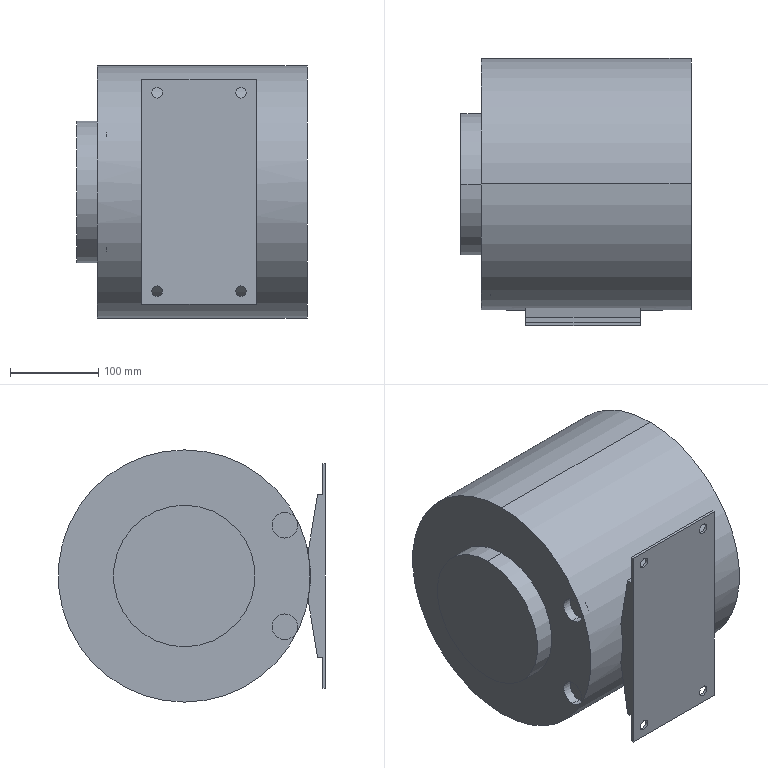Part | SolidWorks | features BaseBody 1 | 1 solid | 32 faces | box 261 x 303 x 286 mm | volume 16134970 mm3 | cylinder 16 | plane 16 | commonest cylinder face diameters 12 x8 28.835 x4 160.568 x2 286 x2
STEP:
#1=CARTESIAN_POINT('',(10.,-114.,-71.917));
#2=VERTEX_POINT('',#1);
#3=CARTESIAN_POINT('',(10.,-114.,-43.083));
#4=VERTEX_POINT('',#3);
#5=CARTESIAN_POINT('',(10.,-114.,-57.5));
#6=DIRECTION('',(-1.,0.,0.));
#7=DIRECTION('',(0.,0.,-1.));
#8=AXIS2_PLACEMENT_3D('',#5,#6,#7);
#9=CIRCLE('',#8,14.417);
#10=EDGE_CURVE('',#2,#4,#9,.T.);
#11=ORIENTED_EDGE('',*,*,#10,.F.);
#12=CARTESIAN_POINT('',(0.,-114.,-71.917));
#13=VERTEX_POINT('',#12);
#14=CARTESIAN_POINT('',(10.,-114.,-71.917));
#15=DIRECTION('',(-1.,0.,0.));
#16=VECTOR('',#15,1000.);
#17=LINE('',#14,#16);
#18=EDGE_CURVE('',#2,#13,#17,.T.);
#19=ORIENTED_EDGE('',*,*,#18,.T.);
#20=CARTESIAN_POINT('',(0.,-114.,-43.083));
#21=VERTEX_POINT('',#20);
#22=CARTESIAN_POINT('',(0.,-114.,-57.5));
#23=DIRECTION('',(-1.,0.,0.));
#24=DIRECTION('',(0.,0.,-1.));
#25=AXIS2_PLACEMENT_3D('',#22,#23,#24);
#26=CIRCLE('',#25,14.417);
#27=EDGE_CURVE('',#13,#21,#26,.T.);
#28=ORIENTED_EDGE('',*,*,#27,.T.);
#29=CARTESIAN_POINT('',(10.,-114.,-43.083));
#30=DIRECTION('',(-1.,0.,0.));
#31=VECTOR('',#30,1000.);
#32=LINE('',#29,#31);
#33=EDGE_CURVE('',#4,#21,#32,.T.);
#34=ORIENTED_EDGE('',*,*,#33,.F.);
#35=EDGE_LOOP('',(#11,#19,#28,#34));
#36=FACE_OUTER_BOUND('',#35,.T.);
#37=CARTESIAN_POINT('',(10.,-114.,-57.5));
#38=DIRECTION('',(-1.,0.,0.));
#39=DIRECTION('',(0.,0.,1.));
#40=AXIS2_PLACEMENT_3D('',#37,#38,#39);
#41=CYLINDRICAL_SURFACE('',#40,14.417);
#42=ADVANCED_FACE('',(#36),#41,.F.);
#43=CARTESIAN_POINT('',(10.,-114.,43.083));
#44=VERTEX_POINT('',#43);
#45=CARTESIAN_POINT('',(10.,-114.,71.917));
#46=VERTEX_POINT('',#45);
#47=CARTESIAN_POINT('',(10.,-114.,57.5));
#48=DIRECTION('',(-1.,0.,0.));
#49=DIRECTION('',(0.,0.,1.));
#50=AXIS2_PLACEMENT_3D('',#47,#48,#49);
#51=CIRCLE('',#50,14.417);
#52=EDGE_CURVE('',#44,#46,#51,.T.);
#53=ORIENTED_EDGE('',*,*,#52,.F.);
#54=CARTESIAN_POINT('',(0.,-114.,43.083));
#55=VERTEX_POINT('',#54);
#56=CARTESIAN_POINT('',(10.,-114.,43.083));
#57=DIRECTION('',(-1.,0.,0.));
#58=VECTOR('',#57,1000.);
#59=LINE('',#56,#58);
#60=EDGE_CURVE('',#44,#55,#59,.T.);
#61=ORIENTED_EDGE('',*,*,#60,.T.);
#62=CARTESIAN_POINT('',(0.,-114.,71.917));
#63=VERTEX_POINT('',#62);
#64=CARTESIAN_POINT('',(0.,-114.,57.5));
#65=DIRECTION('',(-1.,0.,0.));
#66=DIRECTION('',(0.,0.,1.));
#67=AXIS2_PLACEMENT_3D('',#64,#65,#66);
#68=CIRCLE('',#67,14.417);
#69=EDGE_CURVE('',#55,#63,#68,.T.);
#70=ORIENTED_EDGE('',*,*,#69,.T.);
#71=CARTESIAN_POINT('',(10.,-114.,71.917));
#72=DIRECTION('',(-1.,0.,0.));
#73=VECTOR('',#72,1000.);
#74=LINE('',#71,#73);
#75=EDGE_CURVE('',#46,#63,#74,.T.);
#76=ORIENTED_EDGE('',*,*,#75,.F.);
#77=EDGE_LOOP('',(#53,#61,#70,#76));
#78=FACE_OUTER_BOUND('',#77,.T.);
#79=CARTESIAN_POINT('',(10.,-114.,57.5));
#80=DIRECTION('',(-1.,0.,0.));
#81=DIRECTION('',(0.,0.,1.));
#82=AXIS2_PLACEMENT_3D('',#79,#80,#81);
#83=CYLINDRICAL_SURFACE('',#82,14.417);
#84=ADVANCED_FACE('',(#78),#83,.F.);
#85=CARTESIAN_POINT('',(-23.,0.,80.284));
#86=VERTEX_POINT('',#85);
#87=CARTESIAN_POINT('',(-23.,0.,-80.284));
#88=VERTEX_POINT('',#87);
#89=CARTESIAN_POINT('',(-23.,0.,0.));
#90=DIRECTION('',(-1.,0.,0.));
#91=DIRECTION('',(0.,0.,1.));
#92=AXIS2_PLACEMENT_3D('',#89,#90,#91);
#93=CIRCLE('',#92,80.284);
#94=EDGE_CURVE('',#86,#88,#93,.T.);
#95=ORIENTED_EDGE('',*,*,#94,.F.);
#96=CARTESIAN_POINT('',(0.,0.,80.284));
#97=VERTEX_POINT('',#96);
#98=CARTESIAN_POINT('',(-23.,0.,80.284));
#99=DIRECTION('',(1.,0.,0.));
#100=VECTOR('',#99,1000.);
#101=LINE('',#98,#100);
#102=EDGE_CURVE('',#86,#97,#101,.T.);
#103=ORIENTED_EDGE('',*,*,#102,.T.);
#104=CARTESIAN_POINT('',(0.,0.,-80.284));
#105=VERTEX_POINT('',#104);
#106=CARTESIAN_POINT('',(0.,0.,0.));
#107=DIRECTION('',(-1.,0.,0.));
#108=DIRECTION('',(0.,0.,-1.));
#109=AXIS2_PLACEMENT_3D('',#106,#107,#108);
#110=CIRCLE('',#109,80.284);
#111=EDGE_CURVE('',#97,#105,#110,.T.);
#112=ORIENTED_EDGE('',*,*,#111,.T.);
#113=CARTESIAN_POINT('',(-23.,0.,-80.284));
#114=DIRECTION('',(1.,0.,0.));
#115=VECTOR('',#114,1000.);
#116=LINE('',#113,#115);
#117=EDGE_CURVE('',#88,#105,#116,.T.);
#118=ORIENTED_EDGE('',*,*,#117,.F.);
#119=EDGE_LOOP('',(#95,#103,#112,#118));
#120=FACE_OUTER_BOUND('',#119,.T.);
#121=CARTESIAN_POINT('',(-23.,0.,0.));
#122=DIRECTION('',(1.,0.,0.));
#123=DIRECTION('',(0.,0.,-1.));
#124=AXIS2_PLACEMENT_3D('',#121,#122,#123);
#125=CYLINDRICAL_SURFACE('',#124,80.284);
#126=ADVANCED_FACE('',(#120),#125,.T.);
#127=CARTESIAN_POINT('',(163.,-157.,-106.5));
#128=VERTEX_POINT('',#127);
#129=CARTESIAN_POINT('',(163.,-157.,-118.5));
#130=VERTEX_POINT('',#129);
#131=CARTESIAN_POINT('',(163.,-157.,-112.5));
#132=DIRECTION('',(0.,-1.,0.));
#133=DIRECTION('',(0.,0.,-1.));
#134=AXIS2_PLACEMENT_3D('',#131,#132,#133);
#135=CIRCLE('',#134,6.);
#136=EDGE_CURVE('',#128,#130,#135,.T.);
#137=ORIENTED_EDGE('',*,*,#136,.F.);
#138=CARTESIAN_POINT('',(163.,-160.,-106.5));
#139=VERTEX_POINT('',#138);
#140=CARTESIAN_POINT('',(163.,143.001,-106.5));
#141=DIRECTION('',(0.,-1.,0.));
#142=VECTOR('',#141,1000.);
#143=LINE('',#140,#142);
#144=EDGE_CURVE('',#128,#139,#143,.T.);
#145=ORIENTED_EDGE('',*,*,#144,.T.);
#146=CARTESIAN_POINT('',(163.,-160.,-118.5));
#147=VERTEX_POINT('',#146);
#148=CARTESIAN_POINT('',(163.,-160.,-112.5));
#149=DIRECTION('',(0.,-1.,0.));
#150=DIRECTION('',(0.,0.,-1.));
#151=AXIS2_PLACEMENT_3D('',#148,#149,#150);
#152=CIRCLE('',#151,6.);
#153=EDGE_CURVE('',#139,#147,#152,.T.);
#154=ORIENTED_EDGE('',*,*,#153,.T.);
#155=CARTESIAN_POINT('',(163.,143.001,-118.5));
#156=DIRECTION('',(0.,-1.,0.));
#157=VECTOR('',#156,1000.);
#158=LINE('',#155,#157);
#159=EDGE_CURVE('',#130,#147,#158,.T.);
#160=ORIENTED_EDGE('',*,*,#159,.F.);
#161=EDGE_LOOP('',(#137,#145,#154,#160));
#162=FACE_OUTER_BOUND('',#161,.T.);
#163=CARTESIAN_POINT('',(163.,143.001,-112.5));
#164=DIRECTION('',(0.,-1.,0.));
#165=DIRECTION('',(0.,0.,-1.));
#166=AXIS2_PLACEMENT_3D('',#163,#164,#165);
#167=CYLINDRICAL_SURFACE('',#166,6.);
#168=ADVANCED_FACE('',(#162),#167,.F.);
#169=CARTESIAN_POINT('',(68.,-157.,-106.5));
#170=VERTEX_POINT('',#169);
#171=CARTESIAN_POINT('',(68.,-157.,-118.5));
#172=VERTEX_POINT('',#171);
#173=CARTESIAN_POINT('',(68.,-157.,-112.5));
#174=DIRECTION('',(0.,-1.,0.));
#175=DIRECTION('',(0.,0.,-1.));
#176=AXIS2_PLACEMENT_3D('',#173,#174,#175);
#177=CIRCLE('',#176,6.);
#178=EDGE_CURVE('',#170,#172,#177,.T.);
#179=ORIENTED_EDGE('',*,*,#178,.F.);
#180=CARTESIAN_POINT('',(68.,-160.,-106.5));
#181=VERTEX_POINT('',#180);
#182=CARTESIAN_POINT('',(68.,143.001,-106.5));
#183=DIRECTION('',(0.,-1.,0.));
#184=VECTOR('',#183,1000.);
#185=LINE('',#182,#184);
#186=EDGE_CURVE('',#170,#181,#185,.T.);
#187=ORIENTED_EDGE('',*,*,#186,.T.);
#188=CARTESIAN_POINT('',(68.,-160.,-118.5));
#189=VERTEX_POINT('',#188);
#190=CARTESIAN_POINT('',(68.,-160.,-112.5));
#191=DIRECTION('',(0.,-1.,0.));
#192=DIRECTION('',(0.,0.,1.));
#193=AXIS2_PLACEMENT_3D('',#190,#191,#192);
#194=CIRCLE('',#193,6.);
#195=EDGE_CURVE('',#181,#189,#194,.T.);
#196=ORIENTED_EDGE('',*,*,#195,.T.);
#197=CARTESIAN_POINT('',(68.,143.001,-118.5));
#198=DIRECTION('',(0.,-1.,0.));
#199=VECTOR('',#198,1000.);
#200=LINE('',#197,#199);
#201=EDGE_CURVE('',#172,#189,#200,.T.);
#202=ORIENTED_EDGE('',*,*,#201,.F.);
#203=EDGE_LOOP('',(#179,#187,#196,#202));
#204=FACE_OUTER_BOUND('',#203,.T.);
#205=CARTESIAN_POINT('',(68.,143.001,-112.5));
#206=DIRECTION('',(0.,-1.,0.));
#207=DIRECTION('',(0.,0.,-1.));
#208=AXIS2_PLACEMENT_3D('',#205,#206,#207);
#209=CYLINDRICAL_SURFACE('',#208,6.);
#210=ADVANCED_FACE('',(#204),#209,.F.);
#211=CARTESIAN_POINT('',(163.,-157.,118.5));
#212=VERTEX_POINT('',#211);
#213=CARTESIAN_POINT('',(163.,-157.,106.5));
#214=VERTEX_POINT('',#213);
#215=CARTESIAN_POINT('',(163.,-157.,112.5));
#216=DIRECTION('',(0.,-1.,0.));
#217=DIRECTION('',(0.,0.,-1.));
#218=AXIS2_PLACEMENT_3D('',#215,#216,#217);
#219=CIRCLE('',#218,6.);
#220=EDGE_CURVE('',#212,#214,#219,.T.);
#221=ORIENTED_EDGE('',*,*,#220,.F.);
#222=CARTESIAN_POINT('',(163.,-160.,118.5));
#223=VERTEX_POINT('',#222);
#224=CARTESIAN_POINT('',(163.,143.001,118.5));
#225=DIRECTION('',(0.,-1.,0.));
#226=VECTOR('',#225,1000.);
#227=LINE('',#224,#226);
#228=EDGE_CURVE('',#212,#223,#227,.T.);
#229=ORIENTED_EDGE('',*,*,#228,.T.);
#230=CARTESIAN_POINT('',(163.,-160.,106.5));
#231=VERTEX_POINT('',#230);
#232=CARTESIAN_POINT('',(163.,-160.,112.5));
#233=DIRECTION('',(0.,-1.,0.));
#234=DIRECTION('',(0.,0.,1.));
#235=AXIS2_PLACEMENT_3D('',#232,#233,#234);
#236=CIRCLE('',#235,6.);
#237=EDGE_CURVE('',#223,#231,#236,.T.);
#238=ORIENTED_EDGE('',*,*,#237,.T.);
#239=CARTESIAN_POINT('',(163.,143.001,106.5));
#240=DIRECTION('',(0.,-1.,0.));
#241=VECTOR('',#240,1000.);
#242=LINE('',#239,#241);
#243=EDGE_CURVE('',#214,#231,#242,.T.);
#244=ORIENTED_EDGE('',*,*,#243,.F.);
#245=EDGE_LOOP('',(#221,#229,#238,#244));
#246=FACE_OUTER_BOUND('',#245,.T.);
#247=CARTESIAN_POINT('',(163.,143.001,112.5));
#248=DIRECTION('',(0.,-1.,0.));
#249=DIRECTION('',(0.,0.,-1.));
#250=AXIS2_PLACEMENT_3D('',#247,#248,#249);
#251=CYLINDRICAL_SURFACE('',#250,6.);
#252=ADVANCED_FACE('',(#246),#251,.F.);
#253=CARTESIAN_POINT('',(68.,-157.,118.5));
#254=VERTEX_POINT('',#253);
#255=CARTESIAN_POINT('',(68.,-157.,106.5));
#256=VERTEX_POINT('',#255);
#257=CARTESIAN_POINT('',(68.,-157.,112.5));
#258=DIRECTION('',(0.,-1.,0.));
#259=DIRECTION('',(0.,0.,-1.));
#260=AXIS2_PLACEMENT_3D('',#257,#258,#259);
#261=CIRCLE('',#260,6.);
#262=EDGE_CURVE('',#254,#256,#261,.T.);
#263=ORIENTED_EDGE('',*,*,#262,.F.);
#264=CARTESIAN_POINT('',(68.,-160.,118.5));
#265=VERTEX_POINT('',#264);
#266=CARTESIAN_POINT('',(68.,143.001,118.5));
#267=DIRECTION('',(0.,-1.,0.));
#268=VECTOR('',#267,1000.);
#269=LINE('',#266,#268);
#270=EDGE_CURVE('',#254,#265,#269,.T.);
#271=ORIENTED_EDGE('',*,*,#270,.T.);
#272=CARTESIAN_POINT('',(68.,-160.,106.5));
#273=VERTEX_POINT('',#272);
#274=CARTESIAN_POINT('',(68.,-160.,112.5));
#275=DIRECTION('',(0.,-1.,0.));
#276=DIRECTION('',(0.,0.,-1.));
#277=AXIS2_PLACEMENT_3D('',#274,#275,#276);
#278=CIRCLE('',#277,6.);
#279=EDGE_CURVE('',#265,#273,#278,.T.);
#280=ORIENTED_EDGE('',*,*,#279,.T.);
#281=CARTESIAN_POINT('',(68.,143.001,106.5));
#282=DIRECTION('',(0.,-1.,0.));
#283=VECTOR('',#282,1000.);
#284=LINE('',#281,#283);
#285=EDGE_CURVE('',#256,#273,#284,.T.);
#286=ORIENTED_EDGE('',*,*,#285,.F.);
#287=EDGE_LOOP('',(#263,#271,#280,#286));
#288=FACE_OUTER_BOUND('',#287,.T.);
#289=CARTESIAN_POINT('',(68.,143.001,112.5));
#290=DIRECTION('',(0.,-1.,0.));
#291=DIRECTION('',(0.,0.,-1.));
#292=AXIS2_PLACEMENT_3D('',#289,#290,#291);
#293=CYLINDRICAL_SURFACE('',#292,6.);
#294=ADVANCED_FACE('',(#288),#293,.F.);
#295=CARTESIAN_POINT('',(238.,0.,-143.));
#296=VERTEX_POINT('',#295);
#297=CARTESIAN_POINT('',(238.,0.,143.));
#298=VERTEX_POINT('',#297);
#299=CARTESIAN_POINT('',(238.,0.,0.));
#300=DIRECTION('',(1.,0.,0.));
#301=DIRECTION('',(0.,0.,-1.));
#302=AXIS2_PLACEMENT_3D('',#299,#300,#301);
#303=CIRCLE('',#302,143.);
#304=EDGE_CURVE('',#296,#298,#303,.T.);
#305=ORIENTED_EDGE('',*,*,#304,.F.);
#306=CARTESIAN_POINT('',(0.,0.,-143.));
#307=VERTEX_POINT('',#306);
#308=CARTESIAN_POINT('',(238.,0.,-143.));
#309=DIRECTION('',(-1.,0.,0.));
#310=VECTOR('',#309,1000.);
#311=LINE('',#308,#310);
#312=EDGE_CURVE('',#296,#307,#311,.T.);
#313=ORIENTED_EDGE('',*,*,#312,.T.);
#314=CARTESIAN_POINT('',(0.,0.,143.));
#315=VERTEX_POINT('',#314);
#316=CARTESIAN_POINT('',(0.,0.,0.));
#317=DIRECTION('',(1.,0.,0.));
#318=DIRECTION('',(0.,0.,-1.));
#319=AXIS2_PLACEMENT_3D('',#316,#317,#318);
#320=CIRCLE('',#319,143.);
#321=EDGE_CURVE('',#307,#315,#320,.T.);
#322=ORIENTED_EDGE('',*,*,#321,.T.);
#323=CARTESIAN_POINT('',(238.,0.,143.));
#324=DIRECTION('',(-1.,0.,0.));
#325=VECTOR('',#324,1000.);
#326=LINE('',#323,#325);
#327=EDGE_CURVE('',#298,#315,#326,.T.);
#328=ORIENTED_EDGE('',*,*,#327,.F.);
#329=EDGE_LOOP('',(#305,#313,#322,#328));
#330=FACE_OUTER_BOUND('',#329,.T.);
#331=CARTESIAN_POINT('',(238.,0.,0.));
#332=DIRECTION('',(-1.,0.,0.));
#333=DIRECTION('',(0.,0.,1.));
#334=AXIS2_PLACEMENT_3D('',#331,#332,#333);
#335=CYLINDRICAL_SURFACE('',#334,143.);
#336=ADVANCED_FACE('',(#330),#335,.T.);
#337=CARTESIAN_POINT('',(50.5,-151.229,92.5));
#338=VERTEX_POINT('',#337);
#339=CARTESIAN_POINT('',(50.5,-157.,92.5));
#340=VERTEX_POINT('',#339);
#341=CARTESIAN_POINT('',(50.5,-157.,92.5));
#342=DIRECTION('',(0.,-1.,0.));
#343=VECTOR('',#342,1000.);
#344=LINE('',#341,#343);
#345=EDGE_CURVE('',#338,#340,#344,.T.);
#346=ORIENTED_EDGE('',*,*,#345,.T.);
#347=CARTESIAN_POINT('',(180.5,-157.,92.5));
#348=VERTEX_POINT('',#347);
#349=CARTESIAN_POINT('',(238.001,-157.,92.5));
#350=DIRECTION('',(-1.,0.,0.));
#351=VECTOR('',#350,1000.);
#352=LINE('',#349,#351);
#353=EDGE_CURVE('',#348,#340,#352,.T.);
#354=ORIENTED_EDGE('',*,*,#353,.F.);
#355=CARTESIAN_POINT('',(180.5,-151.229,92.5));
#356=VERTEX_POINT('',#355);
#357=CARTESIAN_POINT('',(180.5,-157.,92.5));
#358=DIRECTION('',(0.,1.,0.));
#359=VECTOR('',#358,1000.);
#360=LINE('',#357,#359);
#361=EDGE_CURVE('',#348,#356,#360,.T.);
#362=ORIENTED_EDGE('',*,*,#361,.T.);
#363=CARTESIAN_POINT('',(238.001,-151.229,92.5));
#364=DIRECTION('',(1.,0.,0.));
#365=VECTOR('',#364,1000.);
#366=LINE('',#363,#365);
#367=EDGE_CURVE('',#338,#356,#366,.T.);
#368=ORIENTED_EDGE('',*,*,#367,.F.);
#369=EDGE_LOOP('',(#346,#354,#362,#368));
#370=FACE_OUTER_BOUND('',#369,.T.);
#371=CARTESIAN_POINT('',(238.001,-157.,92.5));
#372=DIRECTION('',(0.,0.,-1.));
#373=DIRECTION('',(0.,-1.,0.));
#374=AXIS2_PLACEMENT_3D('',#371,#372,#373);
#375=PLANE('',#374);
#376=ADVANCED_FACE('',(#370),#375,.F.);
#377=CARTESIAN_POINT('',(163.,-157.,112.5));
#378=DIRECTION('',(0.,-1.,0.));
#379=DIRECTION('',(0.,0.,-1.));
#380=AXIS2_PLACEMENT_3D('',#377,#378,#379);
#381=CIRCLE('',#380,6.);
#382=EDGE_CURVE('',#214,#212,#381,.T.);
#383=ORIENTED_EDGE('',*,*,#382,.T.);
#384=ORIENTED_EDGE('',*,*,#220,.T.);
#385=EDGE_LOOP('',(#383,#384));
#386=FACE_BOUND('',#385,.T.);
#387=CARTESIAN_POINT('',(68.,-157.,112.5));
#388=DIRECTION('',(0.,-1.,0.));
#389=DIRECTION('',(0.,0.,-1.));
#390=AXIS2_PLACEMENT_3D('',#387,#388,#389);
#391=CIRCLE('',#390,6.);
#392=EDGE_CURVE('',#256,#254,#391,.T.);
#393=ORIENTED_EDGE('',*,*,#392,.T.);
#394=ORIENTED_EDGE('',*,*,#262,.T.);
#395=EDGE_LOOP('',(#393,#394));
#396=FACE_BOUND('',#395,.T.);
#397=CARTESIAN_POINT('',(180.5,-157.,127.5));
#398=VERTEX_POINT('',#397);
#399=CARTESIAN_POINT('',(180.5,-157.,127.5));
#400=DIRECTION('',(0.,0.,-1.));
#401=VECTOR('',#400,1000.);
#402=LINE('',#399,#401);
#403=EDGE_CURVE('',#398,#348,#402,.T.);
#404=ORIENTED_EDGE('',*,*,#403,.T.);
#405=ORIENTED_EDGE('',*,*,#353,.T.);
#406=CARTESIAN_POINT('',(50.5,-157.,127.5));
#407=VERTEX_POINT('',#406);
#408=CARTESIAN_POINT('',(50.5,-157.,127.5));
#409=DIRECTION('',(0.,0.,1.));
#410=VECTOR('',#409,1000.);
#411=LINE('',#408,#410);
#412=EDGE_CURVE('',#340,#407,#411,.T.);
#413=ORIENTED_EDGE('',*,*,#412,.T.);
#414=CARTESIAN_POINT('',(180.5,-157.,127.5));
#415=DIRECTION('',(-1.,0.,0.));
#416=VECTOR('',#415,1000.);
#417=LINE('',#414,#416);
#418=EDGE_CURVE('',#398,#407,#417,.T.);
#419=ORIENTED_EDGE('',*,*,#418,.F.);
#420=EDGE_LOOP('',(#404,#405,#413,#419));
#421=FACE_OUTER_BOUND('',#420,.T.);
#422=CARTESIAN_POINT('',(238.001,-157.,127.5));
#423=DIRECTION('',(0.,-1.,0.));
#424=DIRECTION('',(-1.,0.,0.));
#425=AXIS2_PLACEMENT_3D('',#422,#423,#424);
#426=PLANE('',#425);
#427=ADVANCED_FACE('',(#386,#396,#421),#426,.F.);
#428=CARTESIAN_POINT('',(180.5,-151.229,-92.5));
#429=VERTEX_POINT('',#428);
#430=CARTESIAN_POINT('',(180.5,-157.,-92.5));
#431=VERTEX_POINT('',#430);
#432=CARTESIAN_POINT('',(180.5,-157.,-92.5));
#433=DIRECTION('',(0.,-1.,0.));
#434=VECTOR('',#433,1000.);
#435=LINE('',#432,#434);
#436=EDGE_CURVE('',#429,#431,#435,.T.);
#437=ORIENTED_EDGE('',*,*,#436,.T.);
#438=CARTESIAN_POINT('',(50.5,-157.,-92.5));
#439=VERTEX_POINT('',#438);
#440=CARTESIAN_POINT('',(238.001,-157.,-92.5));
#441=DIRECTION('',(-1.,0.,0.));
#442=VECTOR('',#441,1000.);
#443=LINE('',#440,#442);
#444=EDGE_CURVE('',#431,#439,#443,.T.);
#445=ORIENTED_EDGE('',*,*,#444,.T.);
#446=CARTESIAN_POINT('',(50.5,-151.229,-92.5));
#447=VERTEX_POINT('',#446);
#448=CARTESIAN_POINT('',(50.5,-157.,-92.5));
#449=DIRECTION('',(0.,1.,0.));
#450=VECTOR('',#449,1000.);
#451=LINE('',#448,#450);
#452=EDGE_CURVE('',#439,#447,#451,.T.);
#453=ORIENTED_EDGE('',*,*,#452,.T.);
#454=CARTESIAN_POINT('',(238.001,-151.229,-92.5));
#455=DIRECTION('',(-1.,0.,0.));
#456=VECTOR('',#455,1000.);
#457=LINE('',#454,#456);
#458=EDGE_CURVE('',#429,#447,#457,.T.);
#459=ORIENTED_EDGE('',*,*,#458,.F.);
#460=EDGE_LOOP('',(#437,#445,#453,#459));
#461=FACE_OUTER_BOUND('',#460,.T.);
#462=CARTESIAN_POINT('',(238.001,-157.,-92.5));
#463=DIRECTION('',(0.,0.,1.));
#464=DIRECTION('',(1.,0.,0.));
#465=AXIS2_PLACEMENT_3D('',#462,#463,#464);
#466=PLANE('',#465);
#467=ADVANCED_FACE('',(#461),#466,.F.);
#468=CARTESIAN_POINT('',(163.,-157.,-112.5));
#469=DIRECTION('',(0.,-1.,0.));
#470=DIRECTION('',(0.,0.,-1.));
#471=AXIS2_PLACEMENT_3D('',#468,#469,#470);
#472=CIRCLE('',#471,6.);
#473=EDGE_CURVE('',#130,#128,#472,.T.);
#474=ORIENTED_EDGE('',*,*,#473,.T.);
#475=ORIENTED_EDGE('',*,*,#136,.T.);
#476=EDGE_LOOP('',(#474,#475));
#477=FACE_BOUND('',#476,.T.);
#478=CARTESIAN_POINT('',(68.,-157.,-112.5));
#479=DIRECTION('',(0.,-1.,0.));
#480=DIRECTION('',(0.,0.,-1.));
#481=AXIS2_PLACEMENT_3D('',#478,#479,#480);
#482=CIRCLE('',#481,6.);
#483=EDGE_CURVE('',#172,#170,#482,.T.);
#484=ORIENTED_EDGE('',*,*,#483,.T.);
#485=ORIENTED_EDGE('',*,*,#178,.T.);
#486=EDGE_LOOP('',(#484,#485));
#487=FACE_BOUND('',#486,.T.);
#488=CARTESIAN_POINT('',(180.5,-157.,-127.5));
#489=VERTEX_POINT('',#488);
#490=CARTESIAN_POINT('',(180.5,-157.,-127.5));
#491=DIRECTION('',(0.,0.,-1.));
#492=VECTOR('',#491,1000.);
#493=LINE('',#490,#492);
#494=EDGE_CURVE('',#431,#489,#493,.T.);
#495=ORIENTED_EDGE('',*,*,#494,.T.);
#496=CARTESIAN_POINT('',(50.5,-157.,-127.5));
#497=VERTEX_POINT('',#496);
#498=CARTESIAN_POINT('',(180.5,-157.,-127.5));
#499=DIRECTION('',(-1.,0.,0.));
#500=VECTOR('',#499,1000.);
#501=LINE('',#498,#500);
#502=EDGE_CURVE('',#489,#497,#501,.T.);
#503=ORIENTED_EDGE('',*,*,#502,.T.);
#504=CARTESIAN_POINT('',(50.5,-157.,-127.5));
#505=DIRECTION('',(0.,0.,1.));
#506=VECTOR('',#505,1000.);
#507=LINE('',#504,#506);
#508=EDGE_CURVE('',#497,#439,#507,.T.);
#509=ORIENTED_EDGE('',*,*,#508,.T.);
#510=ORIENTED_EDGE('',*,*,#444,.F.);
#511=EDGE_LOOP('',(#495,#503,#509,#510));
#512=FACE_OUTER_BOUND('',#511,.T.);
#513=CARTESIAN_POINT('',(238.001,-157.,-127.5));
#514=DIRECTION('',(0.,-1.,0.));
#515=DIRECTION('',(0.,0.,-1.));
#516=AXIS2_PLACEMENT_3D('',#513,#514,#515);
#517=PLANE('',#516);
#518=ADVANCED_FACE('',(#477,#487,#512),#517,.F.);
#519=CARTESIAN_POINT('',(10.,-114.,-57.5));
#520=DIRECTION('',(-1.,0.,0.));
#521=DIRECTION('',(0.,0.,-1.));
#522=AXIS2_PLACEMENT_3D('',#519,#520,#521);
#523=CIRCLE('',#522,14.417);
#524=EDGE_CURVE('',#4,#2,#523,.T.);
#525=ORIENTED_EDGE('',*,*,#524,.T.);
#526=ORIENTED_EDGE('',*,*,#10,.T.);
#527=EDGE_LOOP('',(#525,#526));
#528=FACE_OUTER_BOUND('',#527,.T.);
#529=CARTESIAN_POINT('',(10.,-114.,-57.5));
#530=DIRECTION('',(1.,0.,0.));
#531=DIRECTION('',(0.,1.,0.));
#532=AXIS2_PLACEMENT_3D('',#529,#530,#531);
#533=PLANE('',#532);
#534=ADVANCED_FACE('',(#528),#533,.F.);
#535=CARTESIAN_POINT('',(10.,-114.,57.5));
#536=DIRECTION('',(-1.,0.,0.));
#537=DIRECTION('',(0.,0.,1.));
#538=AXIS2_PLACEMENT_3D('',#535,#536,#537);
#539=CIRCLE('',#538,14.417);
#540=EDGE_CURVE('',#46,#44,#539,.T.);
#541=ORIENTED_EDGE('',*,*,#540,.T.);
#542=ORIENTED_EDGE('',*,*,#52,.T.);
#543=EDGE_LOOP('',(#541,#542));
#544=FACE_OUTER_BOUND('',#543,.T.);
#545=CARTESIAN_POINT('',(10.,-114.,57.5));
#546=DIRECTION('',(-1.,0.,0.));
#547=DIRECTION('',(0.,0.,1.));
#548=AXIS2_PLACEMENT_3D('',#545,#546,#547);
#549=PLANE('',#548);
#550=ADVANCED_FACE('',(#544),#549,.T.);
#551=CARTESIAN_POINT('',(-23.,0.,0.));
#552=DIRECTION('',(-1.,0.,0.));
#553=DIRECTION('',(0.,0.,1.));
#554=AXIS2_PLACEMENT_3D('',#551,#552,#553);
#555=CIRCLE('',#554,80.284);
#556=EDGE_CURVE('',#88,#86,#555,.T.);
#557=ORIENTED_EDGE('',*,*,#556,.T.);
#558=ORIENTED_EDGE('',*,*,#94,.T.);
#559=EDGE_LOOP('',(#557,#558));
#560=FACE_OUTER_BOUND('',#559,.T.);
#561=CARTESIAN_POINT('',(-23.,0.,0.));
#562=DIRECTION('',(-1.,0.,0.));
#563=DIRECTION('',(0.,0.,1.));
#564=AXIS2_PLACEMENT_3D('',#561,#562,#563);
#565=PLANE('',#564);
#566=ADVANCED_FACE('',(#560),#565,.T.);
#567=ORIENTED_EDGE('',*,*,#412,.F.);
#568=ORIENTED_EDGE('',*,*,#345,.F.);
#569=CARTESIAN_POINT('',(50.5,-140.429,26.995));
#570=VERTEX_POINT('',#569);
#571=CARTESIAN_POINT('',(50.5,-157.,127.5));
#572=DIRECTION('',(0.,0.1627,-0.9867));
#573=VECTOR('',#572,1000.);
#574=LINE('',#571,#573);
#575=EDGE_CURVE('',#338,#570,#574,.T.);
#576=ORIENTED_EDGE('',*,*,#575,.T.);
#577=CARTESIAN_POINT('',(50.5,-140.429,-26.995));
#578=VERTEX_POINT('',#577);
#579=CARTESIAN_POINT('',(50.5,0.,0.));
#580=DIRECTION('',(1.,0.,0.));
#581=DIRECTION('',(0.,0.,1.));
#582=AXIS2_PLACEMENT_3D('',#579,#580,#581);
#583=CIRCLE('',#582,143.);
#584=EDGE_CURVE('',#570,#578,#583,.T.);
#585=ORIENTED_EDGE('',*,*,#584,.T.);
#586=CARTESIAN_POINT('',(50.5,-157.,-127.5));
#587=DIRECTION('',(0.,-0.1627,-0.9867));
#588=VECTOR('',#587,1000.);
#589=LINE('',#586,#588);
#590=EDGE_CURVE('',#578,#447,#589,.T.);
#591=ORIENTED_EDGE('',*,*,#590,.T.);
#592=ORIENTED_EDGE('',*,*,#452,.F.);
#593=ORIENTED_EDGE('',*,*,#508,.F.);
#594=CARTESIAN_POINT('',(50.5,-160.,-127.5));
#595=VERTEX_POINT('',#594);
#596=CARTESIAN_POINT('',(50.5,-160.,-127.5));
#597=DIRECTION('',(0.,-1.,0.));
#598=VECTOR('',#597,1000.);
#599=LINE('',#596,#598);
#600=EDGE_CURVE('',#497,#595,#599,.T.);
#601=ORIENTED_EDGE('',*,*,#600,.T.);
#602=CARTESIAN_POINT('',(50.5,-160.,127.5));
#603=VERTEX_POINT('',#602);
#604=CARTESIAN_POINT('',(50.5,-160.,127.5));
#605=DIRECTION('',(0.,0.,1.));
#606=VECTOR('',#605,1000.);
#607=LINE('',#604,#606);
#608=EDGE_CURVE('',#595,#603,#607,.T.);
#609=ORIENTED_EDGE('',*,*,#608,.T.);
#610=CARTESIAN_POINT('',(50.5,-160.,127.5));
#611=DIRECTION('',(0.,1.,0.));
#612=VECTOR('',#611,1000.);
#613=LINE('',#610,#612);
#614=EDGE_CURVE('',#603,#407,#613,.T.);
#615=ORIENTED_EDGE('',*,*,#614,.T.);
#616=EDGE_LOOP('',(#567,#568,#576,#585,#591,#592,#593,#601,#609,#615));
#617=FACE_OUTER_BOUND('',#616,.T.);
#618=CARTESIAN_POINT('',(50.5,0.,0.));
#619=DIRECTION('',(-1.,0.,0.));
#620=DIRECTION('',(0.,0.,1.));
#621=AXIS2_PLACEMENT_3D('',#618,#619,#620);
#622=PLANE('',#621);
#623=ADVANCED_FACE('',(#617),#622,.T.);
#624=ORIENTED_EDGE('',*,*,#361,.F.);
#625=ORIENTED_EDGE('',*,*,#403,.F.);
#626=CARTESIAN_POINT('',(180.5,-160.,127.5));
#627=VERTEX_POINT('',#626);
#628=CARTESIAN_POINT('',(180.5,-160.,127.5));
#629=DIRECTION('',(0.,1.,0.));
#630=VECTOR('',#629,1000.);
#631=LINE('',#628,#630);
#632=EDGE_CURVE('',#627,#398,#631,.T.);
#633=ORIENTED_EDGE('',*,*,#632,.F.);
#634=CARTESIAN_POINT('',(180.5,-160.,-127.5));
#635=VERTEX_POINT('',#634);
#636=CARTESIAN_POINT('',(180.5,-160.,127.5));
#637=DIRECTION('',(0.,0.,1.));
#638=VECTOR('',#637,1000.);
#639=LINE('',#636,#638);
#640=EDGE_CURVE('',#635,#627,#639,.T.);
#641=ORIENTED_EDGE('',*,*,#640,.F.);
#642=CARTESIAN_POINT('',(180.5,-160.,-127.5));
#643=DIRECTION('',(0.,-1.,0.));
#644=VECTOR('',#643,1000.);
#645=LINE('',#642,#644);
#646=EDGE_CURVE('',#489,#635,#645,.T.);
#647=ORIENTED_EDGE('',*,*,#646,.F.);
#648=ORIENTED_EDGE('',*,*,#494,.F.);
#649=ORIENTED_EDGE('',*,*,#436,.F.);
#650=CARTESIAN_POINT('',(180.5,-140.429,-26.995));
#651=VERTEX_POINT('',#650);
#652=CARTESIAN_POINT('',(180.5,-157.,-127.5));
#653=DIRECTION('',(0.,-0.1627,-0.9867));
#654=VECTOR('',#653,1000.);
#655=LINE('',#652,#654);
#656=EDGE_CURVE('',#651,#429,#655,.T.);
#657=ORIENTED_EDGE('',*,*,#656,.F.);
#658=CARTESIAN_POINT('',(180.5,-140.429,26.995));
#659=VERTEX_POINT('',#658);
#660=CARTESIAN_POINT('',(180.5,0.,0.));
#661=DIRECTION('',(1.,0.,0.));
#662=DIRECTION('',(0.,0.,1.));
#663=AXIS2_PLACEMENT_3D('',#660,#661,#662);
#664=CIRCLE('',#663,143.);
#665=EDGE_CURVE('',#659,#651,#664,.T.);
#666=ORIENTED_EDGE('',*,*,#665,.F.);
#667=CARTESIAN_POINT('',(180.5,-157.,127.5));
#668=DIRECTION('',(0.,0.1627,-0.9867));
#669=VECTOR('',#668,1000.);
#670=LINE('',#667,#669);
#671=EDGE_CURVE('',#356,#659,#670,.T.);
#672=ORIENTED_EDGE('',*,*,#671,.F.);
#673=EDGE_LOOP('',(#624,#625,#633,#641,#647,#648,#649,#657,#666,#672));
#674=FACE_OUTER_BOUND('',#673,.T.);
#675=CARTESIAN_POINT('',(180.5,0.,0.));
#676=DIRECTION('',(-1.,0.,0.));
#677=DIRECTION('',(0.,0.,1.));
#678=AXIS2_PLACEMENT_3D('',#675,#676,#677);
#679=PLANE('',#678);
#680=ADVANCED_FACE('',(#674),#679,.F.);
#681=ORIENTED_EDGE('',*,*,#458,.T.);
#682=ORIENTED_EDGE('',*,*,#590,.F.);
#683=CARTESIAN_POINT('',(180.5,-140.429,-26.995));
#684=DIRECTION('',(-1.,0.,0.));
#685=VECTOR('',#684,1000.);
#686=LINE('',#683,#685);
#687=EDGE_CURVE('',#651,#578,#686,.T.);
#688=ORIENTED_EDGE('',*,*,#687,.F.);
#689=ORIENTED_EDGE('',*,*,#656,.T.);
#690=EDGE_LOOP('',(#681,#682,#688,#689));
#691=FACE_OUTER_BOUND('',#690,.T.);
#692=CARTESIAN_POINT('',(180.5,-157.,-127.5));
#693=DIRECTION('',(0.,0.9867,-0.1627));
#694=DIRECTION('',(-1.,0.,0.));
#695=AXIS2_PLACEMENT_3D('',#692,#693,#694);
#696=PLANE('',#695);
#697=ADVANCED_FACE('',(#691),#696,.T.);
#698=ORIENTED_EDGE('',*,*,#600,.F.);
#699=ORIENTED_EDGE('',*,*,#502,.F.);
#700=ORIENTED_EDGE('',*,*,#646,.T.);
#701=CARTESIAN_POINT('',(180.5,-160.,-127.5));
#702=DIRECTION('',(-1.,0.,0.));
#703=VECTOR('',#702,1000.);
#704=LINE('',#701,#703);
#705=EDGE_CURVE('',#635,#595,#704,.T.);
#706=ORIENTED_EDGE('',*,*,#705,.T.);
#707=EDGE_LOOP('',(#698,#699,#700,#706));
#708=FACE_OUTER_BOUND('',#707,.T.);
#709=CARTESIAN_POINT('',(180.5,-160.,-127.5));
#710=DIRECTION('',(0.,0.,-1.));
#711=DIRECTION('',(0.,-1.,0.));
#712=AXIS2_PLACEMENT_3D('',#709,#710,#711);
#713=PLANE('',#712);
#714=ADVANCED_FACE('',(#708),#713,.T.);
#715=CARTESIAN_POINT('',(68.,-160.,112.5));
#716=DIRECTION('',(0.,-1.,0.));
#717=DIRECTION('',(0.,0.,-1.));
#718=AXIS2_PLACEMENT_3D('',#715,#716,#717);
#719=CIRCLE('',#718,6.);
#720=EDGE_CURVE('',#273,#265,#719,.T.);
#721=ORIENTED_EDGE('',*,*,#720,.F.);
#722=ORIENTED_EDGE('',*,*,#279,.F.);
#723=EDGE_LOOP('',(#721,#722));
#724=FACE_BOUND('',#723,.T.);
#725=CARTESIAN_POINT('',(163.,-160.,112.5));
#726=DIRECTION('',(0.,-1.,0.));
#727=DIRECTION('',(0.,0.,1.));
#728=AXIS2_PLACEMENT_3D('',#725,#726,#727);
#729=CIRCLE('',#728,6.);
#730=EDGE_CURVE('',#231,#223,#729,.T.);
#731=ORIENTED_EDGE('',*,*,#730,.F.);
#732=ORIENTED_EDGE('',*,*,#237,.F.);
#733=EDGE_LOOP('',(#731,#732));
#734=FACE_BOUND('',#733,.T.);
#735=CARTESIAN_POINT('',(68.,-160.,-112.5));
#736=DIRECTION('',(0.,-1.,0.));
#737=DIRECTION('',(0.,0.,1.));
#738=AXIS2_PLACEMENT_3D('',#735,#736,#737);
#739=CIRCLE('',#738,6.);
#740=EDGE_CURVE('',#189,#181,#739,.T.);
#741=ORIENTED_EDGE('',*,*,#740,.F.);
#742=ORIENTED_EDGE('',*,*,#195,.F.);
#743=EDGE_LOOP('',(#741,#742));
#744=FACE_BOUND('',#743,.T.);
#745=CARTESIAN_POINT('',(163.,-160.,-112.5));
#746=DIRECTION('',(0.,-1.,0.));
#747=DIRECTION('',(0.,0.,-1.));
#748=AXIS2_PLACEMENT_3D('',#745,#746,#747);
#749=CIRCLE('',#748,6.);
#750=EDGE_CURVE('',#147,#139,#749,.T.);
#751=ORIENTED_EDGE('',*,*,#750,.F.);
#752=ORIENTED_EDGE('',*,*,#153,.F.);
#753=EDGE_LOOP('',(#751,#752));
#754=FACE_BOUND('',#753,.T.);
#755=ORIENTED_EDGE('',*,*,#608,.F.);
#756=ORIENTED_EDGE('',*,*,#705,.F.);
#757=ORIENTED_EDGE('',*,*,#640,.T.);
#758=CARTESIAN_POINT('',(180.5,-160.,127.5));
#759=DIRECTION('',(-1.,0.,0.));
#760=VECTOR('',#759,1000.);
#761=LINE('',#758,#760);
#762=EDGE_CURVE('',#627,#603,#761,.T.);
#763=ORIENTED_EDGE('',*,*,#762,.T.);
#764=EDGE_LOOP('',(#755,#756,#757,#763));
#765=FACE_OUTER_BOUND('',#764,.T.);
#766=CARTESIAN_POINT('',(180.5,-160.,127.5));
#767=DIRECTION('',(0.,-1.,0.));
#768=DIRECTION('',(-1.,0.,0.));
#769=AXIS2_PLACEMENT_3D('',#766,#767,#768);
#770=PLANE('',#769);
#771=ADVANCED_FACE('',(#724,#734,#744,#754,#765),#770,.T.);
#772=ORIENTED_EDGE('',*,*,#614,.F.);
#773=ORIENTED_EDGE('',*,*,#762,.F.);
#774=ORIENTED_EDGE('',*,*,#632,.T.);
#775=ORIENTED_EDGE('',*,*,#418,.T.);
#776=EDGE_LOOP('',(#772,#773,#774,#775));
#777=FACE_OUTER_BOUND('',#776,.T.);
#778=CARTESIAN_POINT('',(180.5,-160.,127.5));
#779=DIRECTION('',(0.,0.,1.));
#780=DIRECTION('',(1.,0.,0.));
#781=AXIS2_PLACEMENT_3D('',#778,#779,#780);
#782=PLANE('',#781);
#783=ADVANCED_FACE('',(#777),#782,.T.);
#784=ORIENTED_EDGE('',*,*,#367,.T.);
#785=ORIENTED_EDGE('',*,*,#671,.T.);
#786=CARTESIAN_POINT('',(180.5,-140.429,26.995));
#787=DIRECTION('',(-1.,0.,0.));
#788=VECTOR('',#787,1000.);
#789=LINE('',#786,#788);
#790=EDGE_CURVE('',#659,#570,#789,.T.);
#791=ORIENTED_EDGE('',*,*,#790,.T.);
#792=ORIENTED_EDGE('',*,*,#575,.F.);
#793=EDGE_LOOP('',(#784,#785,#791,#792));
#794=FACE_OUTER_BOUND('',#793,.T.);
#795=CARTESIAN_POINT('',(180.5,-157.,127.5));
#796=DIRECTION('',(0.,0.9867,0.1627));
#797=DIRECTION('',(1.,0.,0.));
#798=AXIS2_PLACEMENT_3D('',#795,#796,#797);
#799=PLANE('',#798);
#800=ADVANCED_FACE('',(#794),#799,.T.);
#801=CARTESIAN_POINT('',(238.,0.,0.));
#802=DIRECTION('',(1.,0.,0.));
#803=DIRECTION('',(0.,0.,-1.));
#804=AXIS2_PLACEMENT_3D('',#801,#802,#803);
#805=CIRCLE('',#804,143.);
#806=EDGE_CURVE('',#298,#296,#805,.T.);
#807=ORIENTED_EDGE('',*,*,#806,.T.);
#808=ORIENTED_EDGE('',*,*,#304,.T.);
#809=EDGE_LOOP('',(#807,#808));
#810=FACE_OUTER_BOUND('',#809,.T.);
#811=CARTESIAN_POINT('',(238.,0.,0.));
#812=DIRECTION('',(1.,0.,0.));
#813=DIRECTION('',(0.,1.,0.));
#814=AXIS2_PLACEMENT_3D('',#811,#812,#813);
#815=PLANE('',#814);
#816=ADVANCED_FACE('',(#810),#815,.T.);
#817=CARTESIAN_POINT('',(0.,0.,0.));
#818=DIRECTION('',(-1.,0.,0.));
#819=DIRECTION('',(0.,0.,-1.));
#820=AXIS2_PLACEMENT_3D('',#817,#818,#819);
#821=CIRCLE('',#820,80.284);
#822=EDGE_CURVE('',#105,#97,#821,.T.);
#823=ORIENTED_EDGE('',*,*,#822,.F.);
#824=ORIENTED_EDGE('',*,*,#111,.F.);
#825=EDGE_LOOP('',(#823,#824));
#826=FACE_BOUND('',#825,.T.);
#827=CARTESIAN_POINT('',(0.,-114.,57.5));
#828=DIRECTION('',(-1.,0.,0.));
#829=DIRECTION('',(0.,0.,1.));
#830=AXIS2_PLACEMENT_3D('',#827,#828,#829);
#831=CIRCLE('',#830,14.417);
#832=EDGE_CURVE('',#63,#55,#831,.T.);
#833=ORIENTED_EDGE('',*,*,#832,.F.);
#834=ORIENTED_EDGE('',*,*,#69,.F.);
#835=EDGE_LOOP('',(#833,#834));
#836=FACE_BOUND('',#835,.T.);
#837=CARTESIAN_POINT('',(0.,-114.,-57.5));
#838=DIRECTION('',(-1.,0.,0.));
#839=DIRECTION('',(0.,0.,-1.));
#840=AXIS2_PLACEMENT_3D('',#837,#838,#839);
#841=CIRCLE('',#840,14.417);
#842=EDGE_CURVE('',#21,#13,#841,.T.);
#843=ORIENTED_EDGE('',*,*,#842,.F.);
#844=ORIENTED_EDGE('',*,*,#27,.F.);
#845=EDGE_LOOP('',(#843,#844));
#846=FACE_BOUND('',#845,.T.);
#847=CARTESIAN_POINT('',(0.,0.,0.));
#848=DIRECTION('',(1.,0.,0.));
#849=DIRECTION('',(0.,0.,-1.));
#850=AXIS2_PLACEMENT_3D('',#847,#848,#849);
#851=CIRCLE('',#850,143.);
#852=EDGE_CURVE('',#315,#307,#851,.T.);
#853=ORIENTED_EDGE('',*,*,#852,.F.);
#854=ORIENTED_EDGE('',*,*,#321,.F.);
#855=EDGE_LOOP('',(#853,#854));
#856=FACE_OUTER_BOUND('',#855,.T.);
#857=CARTESIAN_POINT('',(0.,0.,0.));
#858=DIRECTION('',(1.,0.,0.));
#859=DIRECTION('',(0.,1.,0.));
#860=AXIS2_PLACEMENT_3D('',#857,#858,#859);
#861=PLANE('',#860);
#862=ADVANCED_FACE('',(#826,#836,#846,#856),#861,.F.);
#863=ORIENTED_EDGE('',*,*,#312,.F.);
#864=ORIENTED_EDGE('',*,*,#806,.F.);
#865=ORIENTED_EDGE('',*,*,#327,.T.);
#866=ORIENTED_EDGE('',*,*,#852,.T.);
#867=EDGE_LOOP('',(#863,#864,#865,#866));
#868=FACE_OUTER_BOUND('',#867,.T.);
#869=ORIENTED_EDGE('',*,*,#665,.T.);
#870=ORIENTED_EDGE('',*,*,#687,.T.);
#871=ORIENTED_EDGE('',*,*,#584,.F.);
#872=ORIENTED_EDGE('',*,*,#790,.F.);
#873=EDGE_LOOP('',(#869,#870,#871,#872));
#874=FACE_BOUND('',#873,.T.);
#875=CARTESIAN_POINT('',(238.,0.,0.));
#876=DIRECTION('',(-1.,0.,0.));
#877=DIRECTION('',(0.,0.,1.));
#878=AXIS2_PLACEMENT_3D('',#875,#876,#877);
#879=CYLINDRICAL_SURFACE('',#878,143.);
#880=ADVANCED_FACE('',(#868,#874),#879,.T.);
#881=ORIENTED_EDGE('',*,*,#270,.F.);
#882=ORIENTED_EDGE('',*,*,#392,.F.);
#883=ORIENTED_EDGE('',*,*,#285,.T.);
#884=ORIENTED_EDGE('',*,*,#720,.T.);
#885=EDGE_LOOP('',(#881,#882,#883,#884));
#886=FACE_OUTER_BOUND('',#885,.T.);
#887=CARTESIAN_POINT('',(68.,143.001,112.5));
#888=DIRECTION('',(0.,-1.,0.));
#889=DIRECTION('',(0.,0.,-1.));
#890=AXIS2_PLACEMENT_3D('',#887,#888,#889);
#891=CYLINDRICAL_SURFACE('',#890,6.);
#892=ADVANCED_FACE('',(#886),#891,.F.);
#893=ORIENTED_EDGE('',*,*,#228,.F.);
#894=ORIENTED_EDGE('',*,*,#382,.F.);
#895=ORIENTED_EDGE('',*,*,#243,.T.);
#896=ORIENTED_EDGE('',*,*,#730,.T.);
#897=EDGE_LOOP('',(#893,#894,#895,#896));
#898=FACE_OUTER_BOUND('',#897,.T.);
#899=CARTESIAN_POINT('',(163.,143.001,112.5));
#900=DIRECTION('',(0.,-1.,0.));
#901=DIRECTION('',(0.,0.,-1.));
#902=AXIS2_PLACEMENT_3D('',#899,#900,#901);
#903=CYLINDRICAL_SURFACE('',#902,6.);
#904=ADVANCED_FACE('',(#898),#903,.F.);
#905=ORIENTED_EDGE('',*,*,#186,.F.);
#906=ORIENTED_EDGE('',*,*,#483,.F.);
#907=ORIENTED_EDGE('',*,*,#201,.T.);
#908=ORIENTED_EDGE('',*,*,#740,.T.);
#909=EDGE_LOOP('',(#905,#906,#907,#908));
#910=FACE_OUTER_BOUND('',#909,.T.);
#911=CARTESIAN_POINT('',(68.,143.001,-112.5));
#912=DIRECTION('',(0.,-1.,0.));
#913=DIRECTION('',(0.,0.,-1.));
#914=AXIS2_PLACEMENT_3D('',#911,#912,#913);
#915=CYLINDRICAL_SURFACE('',#914,6.);
#916=ADVANCED_FACE('',(#910),#915,.F.);
#917=ORIENTED_EDGE('',*,*,#144,.F.);
#918=ORIENTED_EDGE('',*,*,#473,.F.);
#919=ORIENTED_EDGE('',*,*,#159,.T.);
#920=ORIENTED_EDGE('',*,*,#750,.T.);
#921=EDGE_LOOP('',(#917,#918,#919,#920));
#922=FACE_OUTER_BOUND('',#921,.T.);
#923=CARTESIAN_POINT('',(163.,143.001,-112.5));
#924=DIRECTION('',(0.,-1.,0.));
#925=DIRECTION('',(0.,0.,-1.));
#926=AXIS2_PLACEMENT_3D('',#923,#924,#925);
#927=CYLINDRICAL_SURFACE('',#926,6.);
#928=ADVANCED_FACE('',(#922),#927,.F.);
#929=ORIENTED_EDGE('',*,*,#102,.F.);
#930=ORIENTED_EDGE('',*,*,#556,.F.);
#931=ORIENTED_EDGE('',*,*,#117,.T.);
#932=ORIENTED_EDGE('',*,*,#822,.T.);
#933=EDGE_LOOP('',(#929,#930,#931,#932));
#934=FACE_OUTER_BOUND('',#933,.T.);
#935=CARTESIAN_POINT('',(-23.,0.,0.));
#936=DIRECTION('',(1.,0.,0.));
#937=DIRECTION('',(0.,0.,-1.));
#938=AXIS2_PLACEMENT_3D('',#935,#936,#937);
#939=CYLINDRICAL_SURFACE('',#938,80.284);
#940=ADVANCED_FACE('',(#934),#939,.T.);
#941=ORIENTED_EDGE('',*,*,#60,.F.);
#942=ORIENTED_EDGE('',*,*,#540,.F.);
#943=ORIENTED_EDGE('',*,*,#75,.T.);
#944=ORIENTED_EDGE('',*,*,#832,.T.);
#945=EDGE_LOOP('',(#941,#942,#943,#944));
#946=FACE_OUTER_BOUND('',#945,.T.);
#947=CARTESIAN_POINT('',(10.,-114.,57.5));
#948=DIRECTION('',(-1.,0.,0.));
#949=DIRECTION('',(0.,0.,1.));
#950=AXIS2_PLACEMENT_3D('',#947,#948,#949);
#951=CYLINDRICAL_SURFACE('',#950,14.417);
#952=ADVANCED_FACE('',(#946),#951,.F.);
#953=ORIENTED_EDGE('',*,*,#18,.F.);
#954=ORIENTED_EDGE('',*,*,#524,.F.);
#955=ORIENTED_EDGE('',*,*,#33,.T.);
#956=ORIENTED_EDGE('',*,*,#842,.T.);
#957=EDGE_LOOP('',(#953,#954,#955,#956));
#958=FACE_OUTER_BOUND('',#957,.T.);
#959=CARTESIAN_POINT('',(10.,-114.,-57.5));
#960=DIRECTION('',(-1.,0.,0.));
#961=DIRECTION('',(0.,0.,1.));
#962=AXIS2_PLACEMENT_3D('',#959,#960,#961);
#963=CYLINDRICAL_SURFACE('',#962,14.417);
#964=ADVANCED_FACE('',(#958),#963,.F.);
#965=CLOSED_SHELL('',(#42,#84,#126,#168,#210,#252,#294,#336,#376,#427,#467,#518,#534,#550,#566,#623,#680,#697,#714,#771,#783,#800,#816,#862,#880,#892,#904,#916,#928,#940,#952,#964));
#966=MANIFOLD_SOLID_BREP('',#965);
#967=CARTESIAN_POINT('',(0.,0.,0.));
#968=DIRECTION('',(0.,0.,1.));
#969=DIRECTION('',(1.,0.,0.));
#970=AXIS2_PLACEMENT_3D('',#967,#968,#969);
#971=(LENGTH_UNIT()NAMED_UNIT(*)SI_UNIT(.MILLI.,.METRE.));
#972=UNCERTAINTY_MEASURE_WITH_UNIT(LENGTH_MEASURE(0.00001),#971,'','');
#973=(NAMED_UNIT(*)PLANE_ANGLE_UNIT()SI_UNIT($,.RADIAN.));
#974=(NAMED_UNIT(*)SI_UNIT($,.STERADIAN.)SOLID_ANGLE_UNIT());
#975=(GEOMETRIC_REPRESENTATION_CONTEXT(3)GLOBAL_UNCERTAINTY_ASSIGNED_CONTEXT((#972))GLOBAL_UNIT_ASSIGNED_CONTEXT((#971,#973,#974))REPRESENTATION_CONTEXT('',''));
#976=ADVANCED_BREP_SHAPE_REPRESENTATION('',(#966,#970),#975);